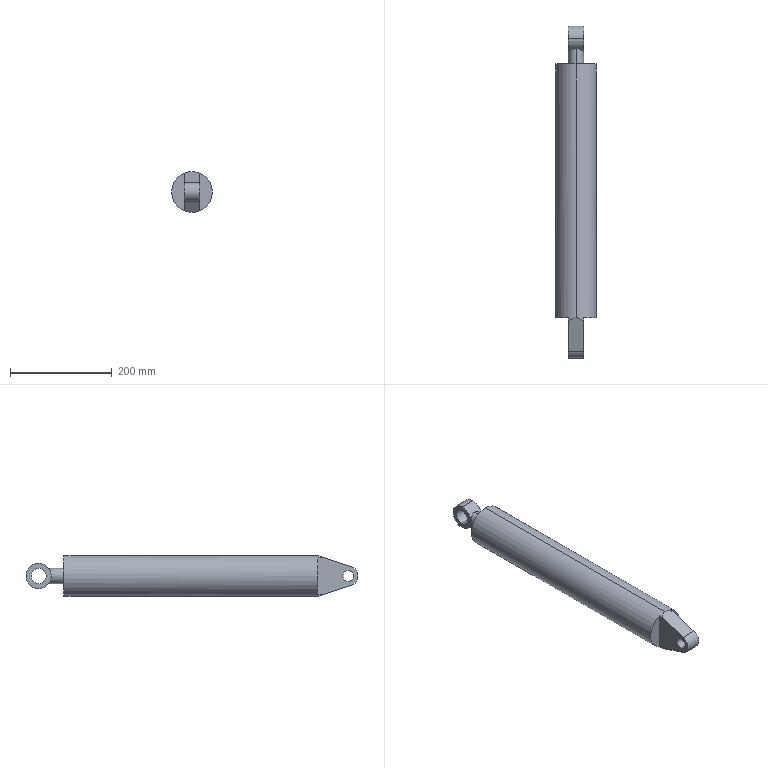Part | SolidWorks | features BaseBody 1 | 1 solid | 21 faces | box 80 x 654.288 x 80 mm | volume 2684074 mm3 | cylinder 12 | plane 9 | commonest cylinder face diameters 30 x4 50 x3 22.047 x2 80 x2 38.577 x1
STEP:
#1=CARTESIAN_POINT('',(15.,550.,-25.));
#2=VERTEX_POINT('',#1);
#3=CARTESIAN_POINT('',(15.,550.,25.));
#4=VERTEX_POINT('',#3);
#5=CARTESIAN_POINT('',(15.,550.,0.));
#6=DIRECTION('',(1.,0.,0.));
#7=DIRECTION('',(0.,0.,-1.));
#8=AXIS2_PLACEMENT_3D('',#5,#6,#7);
#9=CIRCLE('',#8,25.);
#10=EDGE_CURVE('',#2,#4,#9,.T.);
#11=ORIENTED_EDGE('',*,*,#10,.F.);
#12=CARTESIAN_POINT('',(-15.,550.,-25.));
#13=VERTEX_POINT('',#12);
#14=CARTESIAN_POINT('',(15.,550.,-25.));
#15=DIRECTION('',(-1.,0.,0.));
#16=VECTOR('',#15,1000.);
#17=LINE('',#14,#16);
#18=EDGE_CURVE('',#2,#13,#17,.T.);
#19=ORIENTED_EDGE('',*,*,#18,.T.);
#20=CARTESIAN_POINT('',(-15.,550.,25.));
#21=VERTEX_POINT('',#20);
#22=CARTESIAN_POINT('',(-15.,550.,0.));
#23=DIRECTION('',(1.,0.,0.));
#24=DIRECTION('',(0.,0.,-1.));
#25=AXIS2_PLACEMENT_3D('',#22,#23,#24);
#26=CIRCLE('',#25,25.);
#27=EDGE_CURVE('',#13,#21,#26,.T.);
#28=ORIENTED_EDGE('',*,*,#27,.T.);
#29=CARTESIAN_POINT('',(15.,550.,25.));
#30=DIRECTION('',(-1.,0.,0.));
#31=VECTOR('',#30,1000.);
#32=LINE('',#29,#31);
#33=EDGE_CURVE('',#4,#21,#32,.T.);
#34=ORIENTED_EDGE('',*,*,#33,.F.);
#35=EDGE_LOOP('',(#11,#19,#28,#34));
#36=FACE_OUTER_BOUND('',#35,.T.);
#37=CARTESIAN_POINT('',(15.,550.,0.));
#38=DIRECTION('',(-1.,0.,0.));
#39=DIRECTION('',(0.,0.,1.));
#40=AXIS2_PLACEMENT_3D('',#37,#38,#39);
#41=CYLINDRICAL_SURFACE('',#40,25.);
#42=ADVANCED_FACE('',(#36),#41,.T.);
#43=CARTESIAN_POINT('',(15.,525.,0.));
#44=VERTEX_POINT('',#43);
#45=CARTESIAN_POINT('',(15.,550.,0.));
#46=DIRECTION('',(1.,0.,0.));
#47=DIRECTION('',(0.,0.,-1.));
#48=AXIS2_PLACEMENT_3D('',#45,#46,#47);
#49=CIRCLE('',#48,25.);
#50=EDGE_CURVE('',#4,#44,#49,.T.);
#51=ORIENTED_EDGE('',*,*,#50,.F.);
#52=ORIENTED_EDGE('',*,*,#33,.T.);
#53=CARTESIAN_POINT('',(-15.,525.,0.));
#54=VERTEX_POINT('',#53);
#55=CARTESIAN_POINT('',(-15.,550.,0.));
#56=DIRECTION('',(1.,0.,0.));
#57=DIRECTION('',(0.,0.,-1.));
#58=AXIS2_PLACEMENT_3D('',#55,#56,#57);
#59=CIRCLE('',#58,25.);
#60=EDGE_CURVE('',#21,#54,#59,.T.);
#61=ORIENTED_EDGE('',*,*,#60,.T.);
#62=CARTESIAN_POINT('',(0.,530.,15.));
#63=VERTEX_POINT('',#62);
#64=CARTESIAN_POINT('',(0.,530.,15.));
#65=CARTESIAN_POINT('',(-1.019,530.,15.));
#66=CARTESIAN_POINT('',(-2.016,529.922,14.897));
#67=CARTESIAN_POINT('',(-3.482,529.705,14.599));
#68=CARTESIAN_POINT('',(-3.968,529.615,14.474));
#69=CARTESIAN_POINT('',(-4.917,529.41,14.18));
#70=CARTESIAN_POINT('',(-5.379,529.294,14.011));
#71=CARTESIAN_POINT('',(-6.278,529.042,13.632));
#72=CARTESIAN_POINT('',(-6.716,528.906,13.422));
#73=CARTESIAN_POINT('',(-7.569,528.62,12.96));
#74=CARTESIAN_POINT('',(-7.985,528.468,12.707));
#75=CARTESIAN_POINT('',(-9.183,528.005,11.9));
#76=CARTESIAN_POINT('',(-9.919,527.684,11.293));
#77=CARTESIAN_POINT('',(-10.935,527.208,10.279));
#78=CARTESIAN_POINT('',(-11.261,527.049,9.921));
#79=CARTESIAN_POINT('',(-11.876,526.741,9.176));
#80=CARTESIAN_POINT('',(-12.164,526.593,8.791));
#81=CARTESIAN_POINT('',(-12.971,526.167,7.595));
#82=CARTESIAN_POINT('',(-13.434,525.909,6.745));
#83=CARTESIAN_POINT('',(-14.01,525.582,5.382));
#84=CARTESIAN_POINT('',(-14.182,525.482,4.91));
#85=CARTESIAN_POINT('',(-14.476,525.311,3.96));
#86=CARTESIAN_POINT('',(-14.599,525.238,3.479));
#87=CARTESIAN_POINT('',(-14.798,525.121,2.506));
#88=CARTESIAN_POINT('',(-14.873,525.076,2.013));
#89=CARTESIAN_POINT('',(-14.974,525.016,1.016));
#90=CARTESIAN_POINT('',(-15.,525.,0.509));
#91=CARTESIAN_POINT('',(-15.,525.,0.));
#92=B_SPLINE_CURVE_WITH_KNOTS('',3,(#64,#65,#66,#67,#68,#69,#70,#71,#72,#73,#74,#75,#76,#77,#78,#79,#80,#81,#82,#83,#84,#85,#86,#87,#88,#89,#90,#91),.UNSPECIFIED.,.F.,.F.,(4,2,2,2,2,2,2,2,2,2,2,2,2,4),(0.0481,0.05111,0.05261,0.05411,0.05561,0.05711,0.06011,0.06161,0.06311,0.06612,0.06762,0.06912,0.07062,0.07212),.UNSPECIFIED.);
#93=EDGE_CURVE('',#63,#54,#92,.T.);
#94=ORIENTED_EDGE('',*,*,#93,.F.);
#95=CARTESIAN_POINT('',(15.,525.,0.));
#96=CARTESIAN_POINT('',(15.,525.,0.5054));
#97=CARTESIAN_POINT('',(14.974,525.016,1.016));
#98=CARTESIAN_POINT('',(14.872,525.076,2.017));
#99=CARTESIAN_POINT('',(14.797,525.122,2.512));
#100=CARTESIAN_POINT('',(14.597,525.24,3.488));
#101=CARTESIAN_POINT('',(14.473,525.313,3.971));
#102=CARTESIAN_POINT('',(14.177,525.485,4.924));
#103=CARTESIAN_POINT('',(14.005,525.584,5.394));
#104=CARTESIAN_POINT('',(13.43,525.912,6.754));
#105=CARTESIAN_POINT('',(12.964,526.17,7.608));
#106=CARTESIAN_POINT('',(12.146,526.602,8.815));
#107=CARTESIAN_POINT('',(11.855,526.752,9.203));
#108=CARTESIAN_POINT('',(11.242,527.059,9.942));
#109=CARTESIAN_POINT('',(10.92,527.215,10.295));
#110=CARTESIAN_POINT('',(10.244,527.531,10.968));
#111=CARTESIAN_POINT('',(9.89,527.691,11.288));
#112=CARTESIAN_POINT('',(9.149,528.009,11.896));
#113=CARTESIAN_POINT('',(8.76,528.169,12.186));
#114=CARTESIAN_POINT('',(7.563,528.63,12.989));
#115=CARTESIAN_POINT('',(6.72,528.919,13.446));
#116=CARTESIAN_POINT('',(5.379,529.294,14.011));
#117=CARTESIAN_POINT('',(4.919,529.409,14.179));
#118=CARTESIAN_POINT('',(3.97,529.615,14.474));
#119=CARTESIAN_POINT('',(3.484,529.705,14.598));
#120=CARTESIAN_POINT('',(2.018,529.922,14.897));
#121=CARTESIAN_POINT('',(1.019,530.,15.));
#122=CARTESIAN_POINT('',(0.,530.,15.));
#123=B_SPLINE_CURVE_WITH_KNOTS('',3,(#95,#96,#97,#98,#99,#100,#101,#102,#103,#104,#105,#106,#107,#108,#109,#110,#111,#112,#113,#114,#115,#116,#117,#118,#119,#120,#121,#122),.UNSPECIFIED.,.F.,.F.,(4,2,2,2,2,2,2,2,2,2,2,2,2,4),(0.02408,0.02558,0.02708,0.02858,0.03009,0.03309,0.03459,0.03609,0.03759,0.03909,0.0421,0.0436,0.0451,0.0481),.UNSPECIFIED.);
#124=EDGE_CURVE('',#44,#63,#123,.T.);
#125=ORIENTED_EDGE('',*,*,#124,.F.);
#126=EDGE_LOOP('',(#51,#52,#61,#94,#125));
#127=FACE_OUTER_BOUND('',#126,.T.);
#128=CARTESIAN_POINT('',(15.,550.,0.));
#129=DIRECTION('',(-1.,0.,0.));
#130=DIRECTION('',(0.,0.,1.));
#131=AXIS2_PLACEMENT_3D('',#128,#129,#130);
#132=CYLINDRICAL_SURFACE('',#131,25.);
#133=ADVANCED_FACE('',(#127),#132,.T.);
#134=CARTESIAN_POINT('',(15.,550.,15.));
#135=VERTEX_POINT('',#134);
#136=CARTESIAN_POINT('',(15.,550.,-15.));
#137=VERTEX_POINT('',#136);
#138=CARTESIAN_POINT('',(15.,550.,0.));
#139=DIRECTION('',(1.,0.,0.));
#140=DIRECTION('',(0.,0.,-1.));
#141=AXIS2_PLACEMENT_3D('',#138,#139,#140);
#142=CIRCLE('',#141,15.);
#143=EDGE_CURVE('',#135,#137,#142,.T.);
#144=ORIENTED_EDGE('',*,*,#143,.T.);
#145=CARTESIAN_POINT('',(-15.,550.,-15.));
#146=VERTEX_POINT('',#145);
#147=CARTESIAN_POINT('',(15.,550.,-15.));
#148=DIRECTION('',(-1.,0.,0.));
#149=VECTOR('',#148,1000.);
#150=LINE('',#147,#149);
#151=EDGE_CURVE('',#137,#146,#150,.T.);
#152=ORIENTED_EDGE('',*,*,#151,.T.);
#153=CARTESIAN_POINT('',(-15.,550.,15.));
#154=VERTEX_POINT('',#153);
#155=CARTESIAN_POINT('',(-15.,550.,0.));
#156=DIRECTION('',(1.,0.,0.));
#157=DIRECTION('',(0.,0.,-1.));
#158=AXIS2_PLACEMENT_3D('',#155,#156,#157);
#159=CIRCLE('',#158,15.);
#160=EDGE_CURVE('',#154,#146,#159,.T.);
#161=ORIENTED_EDGE('',*,*,#160,.F.);
#162=CARTESIAN_POINT('',(15.,550.,15.));
#163=DIRECTION('',(-1.,0.,0.));
#164=VECTOR('',#163,1000.);
#165=LINE('',#162,#164);
#166=EDGE_CURVE('',#135,#154,#165,.T.);
#167=ORIENTED_EDGE('',*,*,#166,.F.);
#168=EDGE_LOOP('',(#144,#152,#161,#167));
#169=FACE_OUTER_BOUND('',#168,.T.);
#170=CARTESIAN_POINT('',(15.,550.,0.));
#171=DIRECTION('',(-1.,0.,0.));
#172=DIRECTION('',(0.,0.,1.));
#173=AXIS2_PLACEMENT_3D('',#170,#171,#172);
#174=CYLINDRICAL_SURFACE('',#173,15.);
#175=ADVANCED_FACE('',(#169),#174,.F.);
#176=CARTESIAN_POINT('',(15.,-60.,11.023));
#177=VERTEX_POINT('',#176);
#178=CARTESIAN_POINT('',(15.,-60.,-11.023));
#179=VERTEX_POINT('',#178);
#180=CARTESIAN_POINT('',(15.,-60.,0.));
#181=DIRECTION('',(1.,0.,0.));
#182=DIRECTION('',(0.,0.,-1.));
#183=AXIS2_PLACEMENT_3D('',#180,#181,#182);
#184=CIRCLE('',#183,11.023);
#185=EDGE_CURVE('',#177,#179,#184,.T.);
#186=ORIENTED_EDGE('',*,*,#185,.T.);
#187=CARTESIAN_POINT('',(-15.,-60.,-11.023));
#188=VERTEX_POINT('',#187);
#189=CARTESIAN_POINT('',(15.,-60.,-11.023));
#190=DIRECTION('',(-1.,0.,0.));
#191=VECTOR('',#190,1000.);
#192=LINE('',#189,#191);
#193=EDGE_CURVE('',#179,#188,#192,.T.);
#194=ORIENTED_EDGE('',*,*,#193,.T.);
#195=CARTESIAN_POINT('',(-15.,-60.,11.023));
#196=VERTEX_POINT('',#195);
#197=CARTESIAN_POINT('',(-15.,-60.,0.));
#198=DIRECTION('',(1.,0.,0.));
#199=DIRECTION('',(0.,0.,-1.));
#200=AXIS2_PLACEMENT_3D('',#197,#198,#199);
#201=CIRCLE('',#200,11.023);
#202=EDGE_CURVE('',#196,#188,#201,.T.);
#203=ORIENTED_EDGE('',*,*,#202,.F.);
#204=CARTESIAN_POINT('',(15.,-60.,11.023));
#205=DIRECTION('',(-1.,0.,0.));
#206=VECTOR('',#205,1000.);
#207=LINE('',#204,#206);
#208=EDGE_CURVE('',#177,#196,#207,.T.);
#209=ORIENTED_EDGE('',*,*,#208,.F.);
#210=EDGE_LOOP('',(#186,#194,#203,#209));
#211=FACE_OUTER_BOUND('',#210,.T.);
#212=CARTESIAN_POINT('',(15.,-60.,0.));
#213=DIRECTION('',(-1.,0.,0.));
#214=DIRECTION('',(0.,0.,1.));
#215=AXIS2_PLACEMENT_3D('',#212,#213,#214);
#216=CYLINDRICAL_SURFACE('',#215,11.023);
#217=ADVANCED_FACE('',(#211),#216,.F.);
#218=CARTESIAN_POINT('',(0.,500.,40.));
#219=VERTEX_POINT('',#218);
#220=CARTESIAN_POINT('',(0.,500.,-40.));
#221=VERTEX_POINT('',#220);
#222=CARTESIAN_POINT('',(0.,500.,0.));
#223=DIRECTION('',(0.,1.,0.));
#224=DIRECTION('',(0.,0.,1.));
#225=AXIS2_PLACEMENT_3D('',#222,#223,#224);
#226=CIRCLE('',#225,40.);
#227=EDGE_CURVE('',#219,#221,#226,.T.);
#228=ORIENTED_EDGE('',*,*,#227,.F.);
#229=CARTESIAN_POINT('',(0.,0.,40.));
#230=VERTEX_POINT('',#229);
#231=CARTESIAN_POINT('',(0.,500.,40.));
#232=DIRECTION('',(0.,-1.,0.));
#233=VECTOR('',#232,1000.);
#234=LINE('',#231,#233);
#235=EDGE_CURVE('',#219,#230,#234,.T.);
#236=ORIENTED_EDGE('',*,*,#235,.T.);
#237=CARTESIAN_POINT('',(15.,-8.891,37.081));
#238=VERTEX_POINT('',#237);
#239=CARTESIAN_POINT('',(0.,0.,40.));
#240=CARTESIAN_POINT('',(5.157,0.,40.));
#241=CARTESIAN_POINT('',(10.219,-3.,39.015));
#242=CARTESIAN_POINT('',(15.,-8.891,37.081));
#243=(BOUNDED_CURVE()B_SPLINE_CURVE(3,(#239,#240,#241,#242),.UNSPECIFIED.,.F.,.F.)B_SPLINE_CURVE_WITH_KNOTS((4,4),(3.142,3.526),.UNSPECIFIED.)CURVE()GEOMETRIC_REPRESENTATION_ITEM()RATIONAL_B_SPLINE_CURVE((1.,0.9877,0.9877,1.))REPRESENTATION_ITEM(''));
#244=EDGE_CURVE('',#230,#238,#243,.T.);
#245=ORIENTED_EDGE('',*,*,#244,.T.);
#246=CARTESIAN_POINT('',(15.,0.,37.081));
#247=VERTEX_POINT('',#246);
#248=CARTESIAN_POINT('',(15.,575.,37.081));
#249=DIRECTION('',(0.,-1.,0.));
#250=VECTOR('',#249,1000.);
#251=LINE('',#248,#250);
#252=EDGE_CURVE('',#247,#238,#251,.T.);
#253=ORIENTED_EDGE('',*,*,#252,.F.);
#254=CARTESIAN_POINT('',(15.,0.,-37.081));
#255=VERTEX_POINT('',#254);
#256=CARTESIAN_POINT('',(0.,0.,0.));
#257=DIRECTION('',(0.,1.,0.));
#258=DIRECTION('',(0.,0.,1.));
#259=AXIS2_PLACEMENT_3D('',#256,#257,#258);
#260=CIRCLE('',#259,40.);
#261=EDGE_CURVE('',#247,#255,#260,.T.);
#262=ORIENTED_EDGE('',*,*,#261,.T.);
#263=CARTESIAN_POINT('',(15.,-8.891,-37.081));
#264=VERTEX_POINT('',#263);
#265=CARTESIAN_POINT('',(15.,575.,-37.081));
#266=DIRECTION('',(0.,1.,0.));
#267=VECTOR('',#266,1000.);
#268=LINE('',#265,#267);
#269=EDGE_CURVE('',#264,#255,#268,.T.);
#270=ORIENTED_EDGE('',*,*,#269,.F.);
#271=CARTESIAN_POINT('',(0.,0.,-40.));
#272=VERTEX_POINT('',#271);
#273=CARTESIAN_POINT('',(15.,-8.891,-37.081));
#274=CARTESIAN_POINT('',(10.219,-3.,-39.015));
#275=CARTESIAN_POINT('',(5.157,0.,-40.));
#276=CARTESIAN_POINT('',(0.,0.,-40.));
#277=(BOUNDED_CURVE()B_SPLINE_CURVE(3,(#273,#274,#275,#276),.UNSPECIFIED.,.F.,.F.)B_SPLINE_CURVE_WITH_KNOTS((4,4),(2.757,3.142),.UNSPECIFIED.)CURVE()GEOMETRIC_REPRESENTATION_ITEM()RATIONAL_B_SPLINE_CURVE((1.,0.9877,0.9877,1.))REPRESENTATION_ITEM(''));
#278=EDGE_CURVE('',#264,#272,#277,.T.);
#279=ORIENTED_EDGE('',*,*,#278,.T.);
#280=CARTESIAN_POINT('',(0.,500.,-40.));
#281=DIRECTION('',(0.,-1.,0.));
#282=VECTOR('',#281,1000.);
#283=LINE('',#280,#282);
#284=EDGE_CURVE('',#221,#272,#283,.T.);
#285=ORIENTED_EDGE('',*,*,#284,.F.);
#286=EDGE_LOOP('',(#228,#236,#245,#253,#262,#270,#279,#285));
#287=FACE_OUTER_BOUND('',#286,.T.);
#288=CARTESIAN_POINT('',(0.,500.,0.));
#289=DIRECTION('',(0.,-1.,0.));
#290=DIRECTION('',(0.,0.,-1.));
#291=AXIS2_PLACEMENT_3D('',#288,#289,#290);
#292=CYLINDRICAL_SURFACE('',#291,40.);
#293=ADVANCED_FACE('',(#287),#292,.T.);
#294=ORIENTED_EDGE('',*,*,#124,.T.);
#295=CARTESIAN_POINT('',(0.,500.,15.));
#296=VERTEX_POINT('',#295);
#297=CARTESIAN_POINT('',(0.,500.,15.));
#298=DIRECTION('',(0.,-1.,0.));
#299=VECTOR('',#298,1000.);
#300=LINE('',#297,#299);
#301=EDGE_CURVE('',#63,#296,#300,.T.);
#302=ORIENTED_EDGE('',*,*,#301,.T.);
#303=CARTESIAN_POINT('',(0.,500.,-15.));
#304=VERTEX_POINT('',#303);
#305=CARTESIAN_POINT('',(0.,500.,0.));
#306=DIRECTION('',(0.,-1.,0.));
#307=DIRECTION('',(0.,0.,-1.));
#308=AXIS2_PLACEMENT_3D('',#305,#306,#307);
#309=CIRCLE('',#308,15.);
#310=EDGE_CURVE('',#304,#296,#309,.T.);
#311=ORIENTED_EDGE('',*,*,#310,.F.);
#312=CARTESIAN_POINT('',(0.,530.,-15.));
#313=VERTEX_POINT('',#312);
#314=CARTESIAN_POINT('',(0.,500.,-15.));
#315=DIRECTION('',(0.,-1.,0.));
#316=VECTOR('',#315,1000.);
#317=LINE('',#314,#316);
#318=EDGE_CURVE('',#313,#304,#317,.T.);
#319=ORIENTED_EDGE('',*,*,#318,.F.);
#320=CARTESIAN_POINT('',(0.,530.,-15.));
#321=CARTESIAN_POINT('',(1.021,530.,-15.));
#322=CARTESIAN_POINT('',(2.017,529.922,-14.897));
#323=CARTESIAN_POINT('',(3.479,529.705,-14.599));
#324=CARTESIAN_POINT('',(3.961,529.617,-14.476));
#325=CARTESIAN_POINT('',(4.915,529.41,-14.181));
#326=CARTESIAN_POINT('',(5.377,529.294,-14.012));
#327=CARTESIAN_POINT('',(6.726,528.917,-13.443));
#328=CARTESIAN_POINT('',(7.576,528.626,-12.982));
#329=CARTESIAN_POINT('',(9.183,528.005,-11.9));
#330=CARTESIAN_POINT('',(9.92,527.683,-11.292));
#331=CARTESIAN_POINT('',(10.934,527.208,-10.28));
#332=CARTESIAN_POINT('',(11.257,527.051,-9.926));
#333=CARTESIAN_POINT('',(11.872,526.743,-9.181));
#334=CARTESIAN_POINT('',(12.164,526.593,-8.791));
#335=CARTESIAN_POINT('',(12.974,526.165,-7.589));
#336=CARTESIAN_POINT('',(13.437,525.908,-6.739));
#337=CARTESIAN_POINT('',(14.009,525.582,-5.384));
#338=CARTESIAN_POINT('',(14.179,525.484,-4.919));
#339=CARTESIAN_POINT('',(14.477,525.311,-3.959));
#340=CARTESIAN_POINT('',(14.601,525.238,-3.474));
#341=CARTESIAN_POINT('',(14.898,525.061,-2.008));
#342=CARTESIAN_POINT('',(15.,525.,-1.013));
#343=CARTESIAN_POINT('',(15.,525.,0.));
#344=B_SPLINE_CURVE_WITH_KNOTS('',3,(#320,#321,#322,#323,#324,#325,#326,#327,#328,#329,#330,#331,#332,#333,#334,#335,#336,#337,#338,#339,#340,#341,#342,#343),.UNSPECIFIED.,.F.,.F.,(4,2,2,2,2,2,2,2,2,2,2,4),(0.,0.00301,0.004515,0.00602,0.00903,0.01204,0.01354,0.01505,0.01806,0.01956,0.02107,0.02408),.UNSPECIFIED.);
#345=EDGE_CURVE('',#313,#44,#344,.T.);
#346=ORIENTED_EDGE('',*,*,#345,.T.);
#347=EDGE_LOOP('',(#294,#302,#311,#319,#346));
#348=FACE_OUTER_BOUND('',#347,.T.);
#349=CARTESIAN_POINT('',(0.,500.,0.));
#350=DIRECTION('',(0.,-1.,0.));
#351=DIRECTION('',(0.,0.,-1.));
#352=AXIS2_PLACEMENT_3D('',#349,#350,#351);
#353=CYLINDRICAL_SURFACE('',#352,15.);
#354=ADVANCED_FACE('',(#348),#353,.T.);
#355=ORIENTED_EDGE('',*,*,#185,.F.);
#356=CARTESIAN_POINT('',(15.,-60.,0.));
#357=DIRECTION('',(1.,0.,0.));
#358=DIRECTION('',(0.,0.,-1.));
#359=AXIS2_PLACEMENT_3D('',#356,#357,#358);
#360=CIRCLE('',#359,11.023);
#361=EDGE_CURVE('',#179,#177,#360,.T.);
#362=ORIENTED_EDGE('',*,*,#361,.F.);
#363=EDGE_LOOP('',(#355,#362));
#364=FACE_BOUND('',#363,.T.);
#365=CARTESIAN_POINT('',(15.,0.,40.));
#366=DIRECTION('',(0.,0.,1.));
#367=VECTOR('',#366,1000.);
#368=LINE('',#365,#367);
#369=EDGE_CURVE('',#255,#247,#368,.T.);
#370=ORIENTED_EDGE('',*,*,#369,.T.);
#371=ORIENTED_EDGE('',*,*,#252,.T.);
#372=CARTESIAN_POINT('',(15.,-66.017,18.326));
#373=VERTEX_POINT('',#372);
#374=CARTESIAN_POINT('',(15.,0.,40.));
#375=DIRECTION('',(0.,-0.9501,-0.3119));
#376=VECTOR('',#375,1000.);
#377=LINE('',#374,#376);
#378=EDGE_CURVE('',#238,#373,#377,.T.);
#379=ORIENTED_EDGE('',*,*,#378,.T.);
#380=CARTESIAN_POINT('',(15.,-66.017,-18.326));
#381=VERTEX_POINT('',#380);
#382=CARTESIAN_POINT('',(15.,-60.,0.));
#383=DIRECTION('',(1.,0.,0.));
#384=DIRECTION('',(0.,0.,-1.));
#385=AXIS2_PLACEMENT_3D('',#382,#383,#384);
#386=CIRCLE('',#385,19.288);
#387=EDGE_CURVE('',#373,#381,#386,.T.);
#388=ORIENTED_EDGE('',*,*,#387,.T.);
#389=CARTESIAN_POINT('',(15.,0.,-40.));
#390=DIRECTION('',(0.,0.9501,-0.3119));
#391=VECTOR('',#390,1000.);
#392=LINE('',#389,#391);
#393=EDGE_CURVE('',#381,#264,#392,.T.);
#394=ORIENTED_EDGE('',*,*,#393,.T.);
#395=ORIENTED_EDGE('',*,*,#269,.T.);
#396=EDGE_LOOP('',(#370,#371,#379,#388,#394,#395));
#397=FACE_OUTER_BOUND('',#396,.T.);
#398=CARTESIAN_POINT('',(15.,-60.,0.));
#399=DIRECTION('',(1.,0.,0.));
#400=DIRECTION('',(0.,0.,-1.));
#401=AXIS2_PLACEMENT_3D('',#398,#399,#400);
#402=PLANE('',#401);
#403=ADVANCED_FACE('',(#364,#397),#402,.T.);
#404=ORIENTED_EDGE('',*,*,#202,.T.);
#405=CARTESIAN_POINT('',(-15.,-60.,0.));
#406=DIRECTION('',(1.,0.,0.));
#407=DIRECTION('',(0.,0.,-1.));
#408=AXIS2_PLACEMENT_3D('',#405,#406,#407);
#409=CIRCLE('',#408,11.023);
#410=EDGE_CURVE('',#188,#196,#409,.T.);
#411=ORIENTED_EDGE('',*,*,#410,.T.);
#412=EDGE_LOOP('',(#404,#411));
#413=FACE_BOUND('',#412,.T.);
#414=CARTESIAN_POINT('',(-15.,0.,37.081));
#415=VERTEX_POINT('',#414);
#416=CARTESIAN_POINT('',(-15.,-8.891,37.081));
#417=VERTEX_POINT('',#416);
#418=CARTESIAN_POINT('',(-15.,575.,37.081));
#419=DIRECTION('',(0.,-1.,0.));
#420=VECTOR('',#419,1000.);
#421=LINE('',#418,#420);
#422=EDGE_CURVE('',#415,#417,#421,.T.);
#423=ORIENTED_EDGE('',*,*,#422,.F.);
#424=CARTESIAN_POINT('',(-15.,0.,-37.081));
#425=VERTEX_POINT('',#424);
#426=CARTESIAN_POINT('',(-15.,0.,40.));
#427=DIRECTION('',(0.,0.,1.));
#428=VECTOR('',#427,1000.);
#429=LINE('',#426,#428);
#430=EDGE_CURVE('',#425,#415,#429,.T.);
#431=ORIENTED_EDGE('',*,*,#430,.F.);
#432=CARTESIAN_POINT('',(-15.,-8.891,-37.081));
#433=VERTEX_POINT('',#432);
#434=CARTESIAN_POINT('',(-15.,575.,-37.081));
#435=DIRECTION('',(0.,1.,0.));
#436=VECTOR('',#435,1000.);
#437=LINE('',#434,#436);
#438=EDGE_CURVE('',#433,#425,#437,.T.);
#439=ORIENTED_EDGE('',*,*,#438,.F.);
#440=CARTESIAN_POINT('',(-15.,-66.017,-18.326));
#441=VERTEX_POINT('',#440);
#442=CARTESIAN_POINT('',(-15.,0.,-40.));
#443=DIRECTION('',(0.,0.9501,-0.3119));
#444=VECTOR('',#443,1000.);
#445=LINE('',#442,#444);
#446=EDGE_CURVE('',#441,#433,#445,.T.);
#447=ORIENTED_EDGE('',*,*,#446,.F.);
#448=CARTESIAN_POINT('',(-15.,-66.017,18.326));
#449=VERTEX_POINT('',#448);
#450=CARTESIAN_POINT('',(-15.,-60.,0.));
#451=DIRECTION('',(1.,0.,0.));
#452=DIRECTION('',(0.,0.,-1.));
#453=AXIS2_PLACEMENT_3D('',#450,#451,#452);
#454=CIRCLE('',#453,19.288);
#455=EDGE_CURVE('',#449,#441,#454,.T.);
#456=ORIENTED_EDGE('',*,*,#455,.F.);
#457=CARTESIAN_POINT('',(-15.,-60.,20.301));
#458=DIRECTION('',(0.,-0.9501,-0.3119));
#459=VECTOR('',#458,1000.);
#460=LINE('',#457,#459);
#461=EDGE_CURVE('',#417,#449,#460,.T.);
#462=ORIENTED_EDGE('',*,*,#461,.F.);
#463=EDGE_LOOP('',(#423,#431,#439,#447,#456,#462));
#464=FACE_OUTER_BOUND('',#463,.T.);
#465=CARTESIAN_POINT('',(-15.,-60.,0.));
#466=DIRECTION('',(1.,0.,0.));
#467=DIRECTION('',(0.,0.,-1.));
#468=AXIS2_PLACEMENT_3D('',#465,#466,#467);
#469=PLANE('',#468);
#470=ADVANCED_FACE('',(#413,#464),#469,.F.);
#471=CARTESIAN_POINT('',(-15.,-8.891,37.081));
#472=CARTESIAN_POINT('',(-10.219,-3.,39.015));
#473=CARTESIAN_POINT('',(-5.157,0.,40.));
#474=CARTESIAN_POINT('',(0.,0.,40.));
#475=(BOUNDED_CURVE()B_SPLINE_CURVE(3,(#471,#472,#473,#474),.UNSPECIFIED.,.F.,.F.)B_SPLINE_CURVE_WITH_KNOTS((4,4),(2.757,3.142),.UNSPECIFIED.)CURVE()GEOMETRIC_REPRESENTATION_ITEM()RATIONAL_B_SPLINE_CURVE((1.,0.9877,0.9877,1.))REPRESENTATION_ITEM(''));
#476=EDGE_CURVE('',#417,#230,#475,.T.);
#477=ORIENTED_EDGE('',*,*,#476,.F.);
#478=ORIENTED_EDGE('',*,*,#461,.T.);
#479=CARTESIAN_POINT('',(15.,-66.017,18.326));
#480=DIRECTION('',(-1.,0.,0.));
#481=VECTOR('',#480,1000.);
#482=LINE('',#479,#481);
#483=EDGE_CURVE('',#373,#449,#482,.T.);
#484=ORIENTED_EDGE('',*,*,#483,.F.);
#485=ORIENTED_EDGE('',*,*,#378,.F.);
#486=ORIENTED_EDGE('',*,*,#244,.F.);
#487=EDGE_LOOP('',(#477,#478,#484,#485,#486));
#488=FACE_OUTER_BOUND('',#487,.T.);
#489=CARTESIAN_POINT('',(15.,-60.,20.301));
#490=DIRECTION('',(0.,0.3119,-0.9501));
#491=DIRECTION('',(0.,0.9501,0.3119));
#492=AXIS2_PLACEMENT_3D('',#489,#490,#491);
#493=PLANE('',#492);
#494=ADVANCED_FACE('',(#488),#493,.F.);
#495=ORIENTED_EDGE('',*,*,#278,.F.);
#496=ORIENTED_EDGE('',*,*,#393,.F.);
#497=CARTESIAN_POINT('',(15.,-66.017,-18.326));
#498=DIRECTION('',(-1.,0.,0.));
#499=VECTOR('',#498,1000.);
#500=LINE('',#497,#499);
#501=EDGE_CURVE('',#381,#441,#500,.T.);
#502=ORIENTED_EDGE('',*,*,#501,.T.);
#503=ORIENTED_EDGE('',*,*,#446,.T.);
#504=CARTESIAN_POINT('',(0.,0.,-40.));
#505=CARTESIAN_POINT('',(-5.157,0.,-40.));
#506=CARTESIAN_POINT('',(-10.219,-3.,-39.015));
#507=CARTESIAN_POINT('',(-15.,-8.891,-37.081));
#508=(BOUNDED_CURVE()B_SPLINE_CURVE(3,(#504,#505,#506,#507),.UNSPECIFIED.,.F.,.T.)B_SPLINE_CURVE_WITH_KNOTS((4,4),(3.142,3.526),.UNSPECIFIED.)CURVE()GEOMETRIC_REPRESENTATION_ITEM()RATIONAL_B_SPLINE_CURVE((1.,0.9877,0.9877,1.))REPRESENTATION_ITEM(''));
#509=EDGE_CURVE('',#272,#433,#508,.T.);
#510=ORIENTED_EDGE('',*,*,#509,.F.);
#511=EDGE_LOOP('',(#495,#496,#502,#503,#510));
#512=FACE_OUTER_BOUND('',#511,.T.);
#513=CARTESIAN_POINT('',(15.,0.,-40.));
#514=DIRECTION('',(0.,0.3119,0.9501));
#515=DIRECTION('',(0.,-0.9501,0.3119));
#516=AXIS2_PLACEMENT_3D('',#513,#514,#515);
#517=PLANE('',#516);
#518=ADVANCED_FACE('',(#512),#517,.F.);
#519=ORIENTED_EDGE('',*,*,#301,.F.);
#520=ORIENTED_EDGE('',*,*,#93,.T.);
#521=CARTESIAN_POINT('',(-15.,525.,0.));
#522=CARTESIAN_POINT('',(-15.,525.,-1.017));
#523=CARTESIAN_POINT('',(-14.898,525.062,-2.015));
#524=CARTESIAN_POINT('',(-14.598,525.239,-3.485));
#525=CARTESIAN_POINT('',(-14.473,525.313,-3.972));
#526=CARTESIAN_POINT('',(-14.176,525.486,-4.928));
#527=CARTESIAN_POINT('',(-14.006,525.584,-5.393));
#528=CARTESIAN_POINT('',(-13.622,525.802,-6.299));
#529=CARTESIAN_POINT('',(-13.41,525.921,-6.739));
#530=CARTESIAN_POINT('',(-12.944,526.178,-7.596));
#531=CARTESIAN_POINT('',(-12.689,526.316,-8.015));
#532=CARTESIAN_POINT('',(-11.87,526.748,-9.223));
#533=CARTESIAN_POINT('',(-11.258,527.057,-9.959));
#534=CARTESIAN_POINT('',(-9.902,527.691,-11.308));
#535=CARTESIAN_POINT('',(-9.151,528.018,-11.924));
#536=CARTESIAN_POINT('',(-7.56,528.631,-12.991));
#537=CARTESIAN_POINT('',(-6.717,528.92,-13.448));
#538=CARTESIAN_POINT('',(-5.366,529.297,-14.016));
#539=CARTESIAN_POINT('',(-4.898,529.414,-14.186));
#540=CARTESIAN_POINT('',(-3.951,529.619,-14.479));
#541=CARTESIAN_POINT('',(-3.472,529.707,-14.601));
#542=CARTESIAN_POINT('',(-2.501,529.85,-14.798));
#543=CARTESIAN_POINT('',(-2.01,529.905,-14.873));
#544=CARTESIAN_POINT('',(-1.014,529.98,-14.974));
#545=CARTESIAN_POINT('',(-0.5086,530.,-15.));
#546=CARTESIAN_POINT('',(0.,530.,-15.));
#547=B_SPLINE_CURVE_WITH_KNOTS('',3,(#521,#522,#523,#524,#525,#526,#527,#528,#529,#530,#531,#532,#533,#534,#535,#536,#537,#538,#539,#540,#541,#542,#543,#544,#545,#546),.UNSPECIFIED.,.F.,.F.,(4,2,2,2,2,2,2,2,2,2,2,2,4),(0.07212,0.07512,0.07662,0.07812,0.07962,0.08112,0.08412,0.08712,0.09012,0.09162,0.09312,0.09462,0.09612),.UNSPECIFIED.);
#548=EDGE_CURVE('',#54,#313,#547,.T.);
#549=ORIENTED_EDGE('',*,*,#548,.T.);
#550=ORIENTED_EDGE('',*,*,#318,.T.);
#551=CARTESIAN_POINT('',(0.,500.,0.));
#552=DIRECTION('',(0.,-1.,0.));
#553=DIRECTION('',(0.,0.,-1.));
#554=AXIS2_PLACEMENT_3D('',#551,#552,#553);
#555=CIRCLE('',#554,15.);
#556=EDGE_CURVE('',#296,#304,#555,.T.);
#557=ORIENTED_EDGE('',*,*,#556,.F.);
#558=EDGE_LOOP('',(#519,#520,#549,#550,#557));
#559=FACE_OUTER_BOUND('',#558,.T.);
#560=CARTESIAN_POINT('',(0.,500.,0.));
#561=DIRECTION('',(0.,-1.,0.));
#562=DIRECTION('',(0.,0.,-1.));
#563=AXIS2_PLACEMENT_3D('',#560,#561,#562);
#564=CYLINDRICAL_SURFACE('',#563,15.);
#565=ADVANCED_FACE('',(#559),#564,.T.);
#566=ORIENTED_EDGE('',*,*,#369,.F.);
#567=ORIENTED_EDGE('',*,*,#261,.F.);
#568=EDGE_LOOP('',(#566,#567));
#569=FACE_OUTER_BOUND('',#568,.T.);
#570=CARTESIAN_POINT('',(0.,0.,0.));
#571=DIRECTION('',(0.,1.,0.));
#572=DIRECTION('',(0.,0.,1.));
#573=AXIS2_PLACEMENT_3D('',#570,#571,#572);
#574=PLANE('',#573);
#575=ADVANCED_FACE('',(#569),#574,.F.);
#576=ORIENTED_EDGE('',*,*,#235,.F.);
#577=CARTESIAN_POINT('',(0.,500.,0.));
#578=DIRECTION('',(0.,1.,0.));
#579=DIRECTION('',(0.,0.,1.));
#580=AXIS2_PLACEMENT_3D('',#577,#578,#579);
#581=CIRCLE('',#580,40.);
#582=EDGE_CURVE('',#221,#219,#581,.T.);
#583=ORIENTED_EDGE('',*,*,#582,.F.);
#584=ORIENTED_EDGE('',*,*,#284,.T.);
#585=ORIENTED_EDGE('',*,*,#509,.T.);
#586=ORIENTED_EDGE('',*,*,#438,.T.);
#587=CARTESIAN_POINT('',(0.,0.,0.));
#588=DIRECTION('',(0.,1.,0.));
#589=DIRECTION('',(0.,0.,1.));
#590=AXIS2_PLACEMENT_3D('',#587,#588,#589);
#591=CIRCLE('',#590,40.);
#592=EDGE_CURVE('',#425,#415,#591,.T.);
#593=ORIENTED_EDGE('',*,*,#592,.T.);
#594=ORIENTED_EDGE('',*,*,#422,.T.);
#595=ORIENTED_EDGE('',*,*,#476,.T.);
#596=EDGE_LOOP('',(#576,#583,#584,#585,#586,#593,#594,#595));
#597=FACE_OUTER_BOUND('',#596,.T.);
#598=CARTESIAN_POINT('',(0.,500.,0.));
#599=DIRECTION('',(0.,-1.,0.));
#600=DIRECTION('',(0.,0.,-1.));
#601=AXIS2_PLACEMENT_3D('',#598,#599,#600);
#602=CYLINDRICAL_SURFACE('',#601,40.);
#603=ADVANCED_FACE('',(#597),#602,.T.);
#604=ORIENTED_EDGE('',*,*,#310,.T.);
#605=ORIENTED_EDGE('',*,*,#556,.T.);
#606=EDGE_LOOP('',(#604,#605));
#607=FACE_BOUND('',#606,.T.);
#608=ORIENTED_EDGE('',*,*,#582,.T.);
#609=ORIENTED_EDGE('',*,*,#227,.T.);
#610=EDGE_LOOP('',(#608,#609));
#611=FACE_OUTER_BOUND('',#610,.T.);
#612=CARTESIAN_POINT('',(0.,500.,0.));
#613=DIRECTION('',(0.,1.,0.));
#614=DIRECTION('',(0.,0.,1.));
#615=AXIS2_PLACEMENT_3D('',#612,#613,#614);
#616=PLANE('',#615);
#617=ADVANCED_FACE('',(#607,#611),#616,.T.);
#618=ORIENTED_EDGE('',*,*,#592,.F.);
#619=ORIENTED_EDGE('',*,*,#430,.T.);
#620=EDGE_LOOP('',(#618,#619));
#621=FACE_OUTER_BOUND('',#620,.T.);
#622=CARTESIAN_POINT('',(0.,0.,0.));
#623=DIRECTION('',(0.,1.,0.));
#624=DIRECTION('',(0.,0.,1.));
#625=AXIS2_PLACEMENT_3D('',#622,#623,#624);
#626=PLANE('',#625);
#627=ADVANCED_FACE('',(#621),#626,.F.);
#628=ORIENTED_EDGE('',*,*,#455,.T.);
#629=ORIENTED_EDGE('',*,*,#501,.F.);
#630=ORIENTED_EDGE('',*,*,#387,.F.);
#631=ORIENTED_EDGE('',*,*,#483,.T.);
#632=EDGE_LOOP('',(#628,#629,#630,#631));
#633=FACE_OUTER_BOUND('',#632,.T.);
#634=CARTESIAN_POINT('',(15.,-60.,0.));
#635=DIRECTION('',(-1.,0.,0.));
#636=DIRECTION('',(0.,0.,1.));
#637=AXIS2_PLACEMENT_3D('',#634,#635,#636);
#638=CYLINDRICAL_SURFACE('',#637,19.288);
#639=ADVANCED_FACE('',(#633),#638,.T.);
#640=ORIENTED_EDGE('',*,*,#193,.F.);
#641=ORIENTED_EDGE('',*,*,#361,.T.);
#642=ORIENTED_EDGE('',*,*,#208,.T.);
#643=ORIENTED_EDGE('',*,*,#410,.F.);
#644=EDGE_LOOP('',(#640,#641,#642,#643));
#645=FACE_OUTER_BOUND('',#644,.T.);
#646=CARTESIAN_POINT('',(15.,-60.,0.));
#647=DIRECTION('',(-1.,0.,0.));
#648=DIRECTION('',(0.,0.,1.));
#649=AXIS2_PLACEMENT_3D('',#646,#647,#648);
#650=CYLINDRICAL_SURFACE('',#649,11.023);
#651=ADVANCED_FACE('',(#645),#650,.F.);
#652=ORIENTED_EDGE('',*,*,#151,.F.);
#653=CARTESIAN_POINT('',(15.,550.,0.));
#654=DIRECTION('',(1.,0.,0.));
#655=DIRECTION('',(0.,0.,-1.));
#656=AXIS2_PLACEMENT_3D('',#653,#654,#655);
#657=CIRCLE('',#656,15.);
#658=EDGE_CURVE('',#137,#135,#657,.T.);
#659=ORIENTED_EDGE('',*,*,#658,.T.);
#660=ORIENTED_EDGE('',*,*,#166,.T.);
#661=CARTESIAN_POINT('',(-15.,550.,0.));
#662=DIRECTION('',(1.,0.,0.));
#663=DIRECTION('',(0.,0.,-1.));
#664=AXIS2_PLACEMENT_3D('',#661,#662,#663);
#665=CIRCLE('',#664,15.);
#666=EDGE_CURVE('',#146,#154,#665,.T.);
#667=ORIENTED_EDGE('',*,*,#666,.F.);
#668=EDGE_LOOP('',(#652,#659,#660,#667));
#669=FACE_OUTER_BOUND('',#668,.T.);
#670=CARTESIAN_POINT('',(15.,550.,0.));
#671=DIRECTION('',(-1.,0.,0.));
#672=DIRECTION('',(0.,0.,1.));
#673=AXIS2_PLACEMENT_3D('',#670,#671,#672);
#674=CYLINDRICAL_SURFACE('',#673,15.);
#675=ADVANCED_FACE('',(#669),#674,.F.);
#676=ORIENTED_EDGE('',*,*,#18,.F.);
#677=CARTESIAN_POINT('',(15.,550.,0.));
#678=DIRECTION('',(1.,0.,0.));
#679=DIRECTION('',(0.,0.,-1.));
#680=AXIS2_PLACEMENT_3D('',#677,#678,#679);
#681=CIRCLE('',#680,25.);
#682=EDGE_CURVE('',#44,#2,#681,.T.);
#683=ORIENTED_EDGE('',*,*,#682,.F.);
#684=ORIENTED_EDGE('',*,*,#345,.F.);
#685=ORIENTED_EDGE('',*,*,#548,.F.);
#686=CARTESIAN_POINT('',(-15.,550.,0.));
#687=DIRECTION('',(1.,0.,0.));
#688=DIRECTION('',(0.,0.,-1.));
#689=AXIS2_PLACEMENT_3D('',#686,#687,#688);
#690=CIRCLE('',#689,25.);
#691=EDGE_CURVE('',#54,#13,#690,.T.);
#692=ORIENTED_EDGE('',*,*,#691,.T.);
#693=EDGE_LOOP('',(#676,#683,#684,#685,#692));
#694=FACE_OUTER_BOUND('',#693,.T.);
#695=CARTESIAN_POINT('',(15.,550.,0.));
#696=DIRECTION('',(-1.,0.,0.));
#697=DIRECTION('',(0.,0.,1.));
#698=AXIS2_PLACEMENT_3D('',#695,#696,#697);
#699=CYLINDRICAL_SURFACE('',#698,25.);
#700=ADVANCED_FACE('',(#694),#699,.T.);
#701=ORIENTED_EDGE('',*,*,#143,.F.);
#702=ORIENTED_EDGE('',*,*,#658,.F.);
#703=EDGE_LOOP('',(#701,#702));
#704=FACE_BOUND('',#703,.T.);
#705=ORIENTED_EDGE('',*,*,#682,.T.);
#706=ORIENTED_EDGE('',*,*,#10,.T.);
#707=ORIENTED_EDGE('',*,*,#50,.T.);
#708=EDGE_LOOP('',(#705,#706,#707));
#709=FACE_OUTER_BOUND('',#708,.T.);
#710=CARTESIAN_POINT('',(15.,0.,0.));
#711=DIRECTION('',(1.,0.,0.));
#712=DIRECTION('',(0.,0.,-1.));
#713=AXIS2_PLACEMENT_3D('',#710,#711,#712);
#714=PLANE('',#713);
#715=ADVANCED_FACE('',(#704,#709),#714,.T.);
#716=ORIENTED_EDGE('',*,*,#160,.T.);
#717=ORIENTED_EDGE('',*,*,#666,.T.);
#718=EDGE_LOOP('',(#716,#717));
#719=FACE_BOUND('',#718,.T.);
#720=ORIENTED_EDGE('',*,*,#691,.F.);
#721=ORIENTED_EDGE('',*,*,#60,.F.);
#722=ORIENTED_EDGE('',*,*,#27,.F.);
#723=EDGE_LOOP('',(#720,#721,#722));
#724=FACE_OUTER_BOUND('',#723,.T.);
#725=CARTESIAN_POINT('',(-15.,0.,0.));
#726=DIRECTION('',(1.,0.,0.));
#727=DIRECTION('',(0.,0.,-1.));
#728=AXIS2_PLACEMENT_3D('',#725,#726,#727);
#729=PLANE('',#728);
#730=ADVANCED_FACE('',(#719,#724),#729,.F.);
#731=CLOSED_SHELL('',(#42,#133,#175,#217,#293,#354,#403,#470,#494,#518,#565,#575,#603,#617,#627,#639,#651,#675,#700,#715,#730));
#732=MANIFOLD_SOLID_BREP('',#731);
#733=CARTESIAN_POINT('',(0.,0.,0.));
#734=DIRECTION('',(0.,0.,1.));
#735=DIRECTION('',(1.,0.,0.));
#736=AXIS2_PLACEMENT_3D('',#733,#734,#735);
#737=(LENGTH_UNIT()NAMED_UNIT(*)SI_UNIT(.MILLI.,.METRE.));
#738=UNCERTAINTY_MEASURE_WITH_UNIT(LENGTH_MEASURE(0.00001),#737,'','');
#739=(NAMED_UNIT(*)PLANE_ANGLE_UNIT()SI_UNIT($,.RADIAN.));
#740=(NAMED_UNIT(*)SI_UNIT($,.STERADIAN.)SOLID_ANGLE_UNIT());
#741=(GEOMETRIC_REPRESENTATION_CONTEXT(3)GLOBAL_UNCERTAINTY_ASSIGNED_CONTEXT((#738))GLOBAL_UNIT_ASSIGNED_CONTEXT((#737,#739,#740))REPRESENTATION_CONTEXT('',''));
#742=ADVANCED_BREP_SHAPE_REPRESENTATION('',(#732,#736),#741);